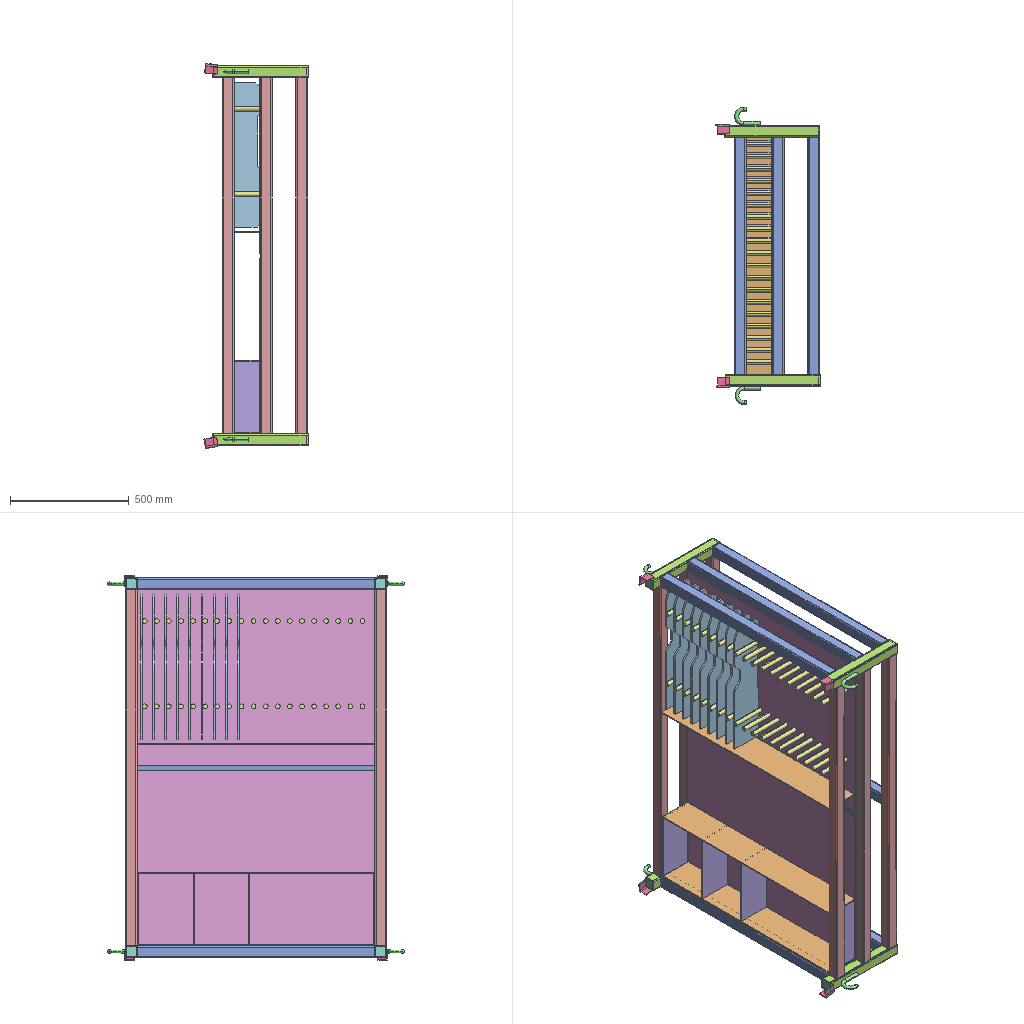Assembly | SolidWorks | 11 different items | 90 placed | box 439 x 1252 x 1625 mm
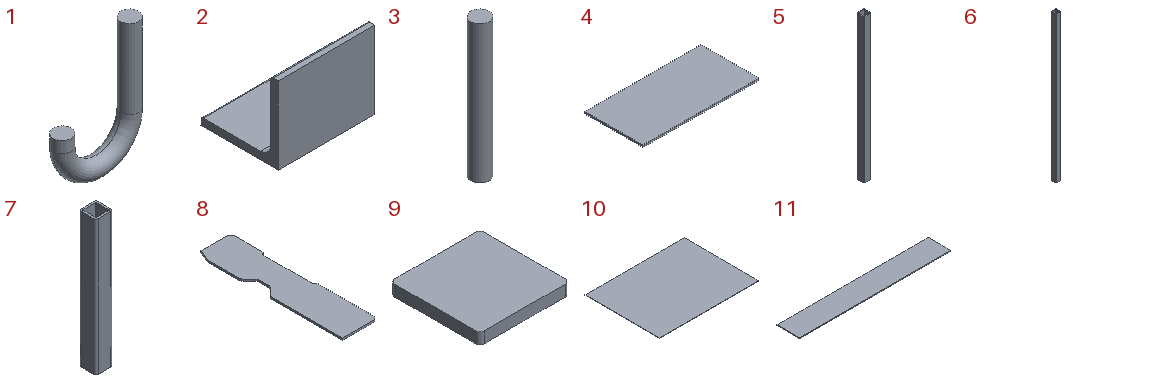Parts list (item | quantity | size | volume | features):
1 | x4 | 76 x 16 x 108 mm | 35035 mm3 | features Sweep 1
2 | x4 | 50 x 40 x 40 mm | 15430 mm3 | features Extrusion 1
3 | x38 | 20 x 20 x 150 mm | 47124 mm3 | features Extrusion 1
4 | x4 | 300 x 150 x 5 mm | 225000 mm3 | features Extrusion 1
5 | x8 | 50 x 50 x 1000 mm | 869956 mm3 | features Extrusion 1
6 | x6 | 50 x 50 x 1500 mm | 1304934 mm3 | features Extrusion 1
7 | x4 | 50 x 50 x 400 mm | 347982 mm3 | features Extrusion 1
8 | x9 | 143 x 607 x 8 mm | 646931 mm3 | features Extrusion 1
9 | x8 | 40 x 40 x 5 mm | 7983 mm3 | features Extrusion 1
10 | x2 | 1000 x 755 x 3 mm | 2265000 mm3 | features Extrusion 1
11 | x3 | 1000 x 150 x 5 mm | 750000 mm3 | features Extrusion 1
Mates (type | each side: item.copy, entity, surface, feature):
Coincident | 6.1 face plane Boss-Extrude1 | 6.2 face plane Boss-Extrude1
Coincident | 6.1 face plane Boss-Extrude1 | 5.1 face plane Boss-Extrude1
Coincident | 6.1 face plane Boss-Extrude1 | 5.2 face plane Boss-Extrude1
Coincident | 5.1 face plane Boss-Extrude1 | 7.1 face plane Boss-Extrude1 | 2 times
Coincident | 6.2 face plane Boss-Extrude1 | 7.1 face plane Boss-Extrude1 | 2 times
Coincident | 6.1 face plane Boss-Extrude1 | 7.2 face plane Boss-Extrude1
Coincident | 5.2 face plane Boss-Extrude1 | 7.2 face plane Boss-Extrude1
Coincident | 7.2 face plane Boss-Extrude1 | 5.3 face plane Boss-Extrude1 | 3 times
DistanceDim | 5.2 face plane Boss-Extrude1 | 5.3 face plane Boss-Extrude1
Coincident | 5.3 face plane Boss-Extrude1 | 5.4 face plane Boss-Extrude1
Coincident | 7.1 face plane Boss-Extrude1 | 5.4 face plane Boss-Extrude1
Coincident | 7.2 face plane Boss-Extrude1 | 6.3 face plane Boss-Extrude1 | 2 times
Coincident | 5.3 face plane Boss-Extrude1 | 6.3 face plane Boss-Extrude1
Coincident | 7.1 face plane Boss-Extrude1 | 6.4 face plane Boss-Extrude1 | 2 times
Coincident | 5.4 face plane Boss-Extrude1 | 6.4 face plane Boss-Extrude1
Coincident | 6.3 face plane Boss-Extrude1 | 5.5 face plane Boss-Extrude1 | 2 times
DistanceDim | 5.5 face plane Boss-Extrude1 | 5.3 face plane Boss-Extrude1
Coincident | 6.2 face plane Boss-Extrude1 | 5.6 face plane Boss-Extrude1 | 2 times
Coincident | 5.5 face plane Boss-Extrude1 | 5.6 face plane Boss-Extrude1
Coincident | 5.2 face plane Boss-Extrude1 | 10.1 face plane Boss-Extrude1
DistanceDim | 10.1 face plane Boss-Extrude1 | 5.2 face plane Boss-Extrude1
Coincident | 10.1 face plane Boss-Extrude1 | 10.2 face plane Boss-Extrude1 | 2 times
DistanceDim | 10.2 face plane Boss-Extrude1 | 5.1 face plane Boss-Extrude1
Parallel | 10.1 face plane Boss-Extrude1 | assembly face | 2 times
Parallel | 6.2 face plane Boss-Extrude1 | assembly face
Coincident | 6.1 face plane Boss-Extrude1 | assembly face
DistanceDim | assembly face | 6.2 face plane Boss-Extrude1
DistanceDim | assembly face | 5.2 face plane Boss-Extrude1
Coincident | 7.1 face plane Boss-Extrude1 | 9.1 face plane Boss-Extrude1 | 3 times
Coincident | 7.1 face plane Boss-Extrude1 | 9.2 face plane Boss-Extrude1 | 3 times
Coincident | 7.2 face plane Boss-Extrude1 | 9.3 face plane Boss-Extrude1 | 3 times
Coincident | 7.2 face plane Boss-Extrude1 | 9.4 face plane Boss-Extrude1 | 3 times
Coincident | assembly face | assembly face | 3 times
Coincident | 7.3 face plane Boss-Extrude1 | 9.5 face plane Boss-Extrude1 | 3 times
Coincident | 7.3 face plane Boss-Extrude1 | 9.6 face plane Boss-Extrude1 | 3 times
Coincident | 9.2 face plane Boss-Extrude1 | 9.6 face plane Boss-Extrude1
Coincident | 6.2 face plane Boss-Extrude1 | 7.3 face plane Boss-Extrude1 | 2 times
Coincident | 7.3 face plane Boss-Extrude1 | 5.3 face plane Boss-Extrude1
Coincident | 5.2 face plane Boss-Extrude1 | 5.3 face plane Boss-Extrude1
Coincident | 6.2 face plane Boss-Extrude1 | 10.1 edge
Coincident | 7.4 face plane Boss-Extrude1 | 11.1 face plane Boss-Extrude1
Coincident | 5.1 face plane Boss-Extrude1 | 11.1 face plane Boss-Extrude1
Coincident | 5.1 face plane Boss-Extrude1 | 7.4 face plane Boss-Extrude1
Coincident | 6.1 face plane Boss-Extrude1 | 7.4 face plane Boss-Extrude1
Coincident | 5.2 face plane Boss-Extrude1 | 7.3 face plane Boss-Extrude1
Coincident | 11.1 face plane Boss-Extrude1 | 11.2 face plane Boss-Extrude1
Coincident | 7.4 face plane Boss-Extrude1 | 11.2 face plane Boss-Extrude1
DistanceDim | 11.2 face plane Boss-Extrude1 | 11.1 face plane Boss-Extrude1
Coincident | 11.1 face plane Boss-Extrude1 | 4.1 face plane Boss-Extrude1 | 2 times
Coincident | 11.2 face plane Boss-Extrude1 | 4.1 face plane Boss-Extrude1
Coincident | 11.2 face plane Boss-Extrude1 | 4.2 face plane Boss-Extrude1 | 3 times
Coincident | 7.2 face plane Boss-Extrude1 | 6.5 face plane Boss-Extrude1 | 2 times
DistanceDim | 6.5 face plane Boss-Extrude1 | 7.2 face plane Boss-Extrude1
Coincident | 6.5 face plane Boss-Extrude1 | 6.6 face plane Boss-Extrude1
Coincident | 7.3 face plane Boss-Extrude1 | 6.6 face plane Boss-Extrude1 | 2 times
Coincident | 6.6 face plane Boss-Extrude1 | 5.7 face plane Boss-Extrude1
Coincident | 7.2 face plane Boss-Extrude1 | 5.7 face plane Boss-Extrude1
Coincident | 7.3 face plane Boss-Extrude1 | 5.7 face plane Boss-Extrude1
Coincident | 6.6 face plane Boss-Extrude1 | 5.8 face plane Boss-Extrude1
Coincident | 7.1 face plane Boss-Extrude1 | 5.8 face plane Boss-Extrude1 | 2 times
Coincident | 11.1 face plane Boss-Extrude1 | 5.8 face plane Boss-Extrude1
Coincident | 11.1 face plane Boss-Extrude1 | 4.3 face plane Boss-Extrude1
Coincident | 11.1 face plane Boss-Extrude1 | 4.4 face plane Boss-Extrude1 | 2 times
Coincident | 11.2 face plane Boss-Extrude1 | 4.3 face plane Boss-Extrude1
Coincident | 7.4 face plane Boss-Extrude1 | 6.3 face plane Boss-Extrude1
Coincident | 7.4 face plane Boss-Extrude1 | 5.4 face plane Boss-Extrude1
Tangent | 1.1 face cylinder Sweep1 | 7.4 face plane Boss-Extrude1
DistanceDim | 1.1 face plane Sweep1 | 7.4 face plane Boss-Extrude1
Parallel | 7.4 face plane Boss-Extrude1 | 1.1 select_type:24
DistanceDim | 1.1 select_type:24 | 7.4 face plane Boss-Extrude1
Tangent | 7.1 face plane Boss-Extrude1 | 1.2 face cylinder Sweep1
DistanceDim | 1.2 face plane Sweep1 | 7.1 face plane Boss-Extrude1
DistanceDim | 1.2 select_type:24 | 7.1 face plane Boss-Extrude1
Tangent | 7.3 face plane Boss-Extrude1 | 1.3 face cylinder Sweep1
DistanceDim | 1.3 face plane Sweep1 | 7.3 face plane Boss-Extrude1
DistanceDim | 1.3 select_type:24 | 7.3 face plane Boss-Extrude1
Tangent | 7.2 face plane Boss-Extrude1 | 1.4 face cylinder Sweep1
DistanceDim | 1.4 face plane Sweep1 | 7.2 face plane Boss-Extrude1
DistanceDim | 1.4 select_type:24 | 7.2 face plane Boss-Extrude1
Coincident | 7.1 face plane Boss-Extrude1 | 2.1 edge | 2 times
Coincident | 7.4 face plane Boss-Extrude1 | 2.2 edge | 2 times
Coincident | 7.2 face plane Boss-Extrude1 | 2.3 edge | 2 times
Coincident | 7.3 face plane Boss-Extrude1 | 2.4 edge | 2 times
Parallel | 6.6 face plane Boss-Extrude1 | assembly face
Coincident | 10.1 face plane Boss-Extrude1 | 8.1 face plane Boss-Extrude1
Parallel | 6.5 face plane Boss-Extrude1 | 8.1 face plane Boss-Extrude1
Coincident | 10.1 face plane Boss-Extrude1 | 3.1 face plane Boss-Extrude1
Coincident | 10.1 face plane Boss-Extrude1 | 11.3 face plane Boss-Extrude1
Coincident | 6.5 face plane Boss-Extrude1 | 11.3 face plane Boss-Extrude1